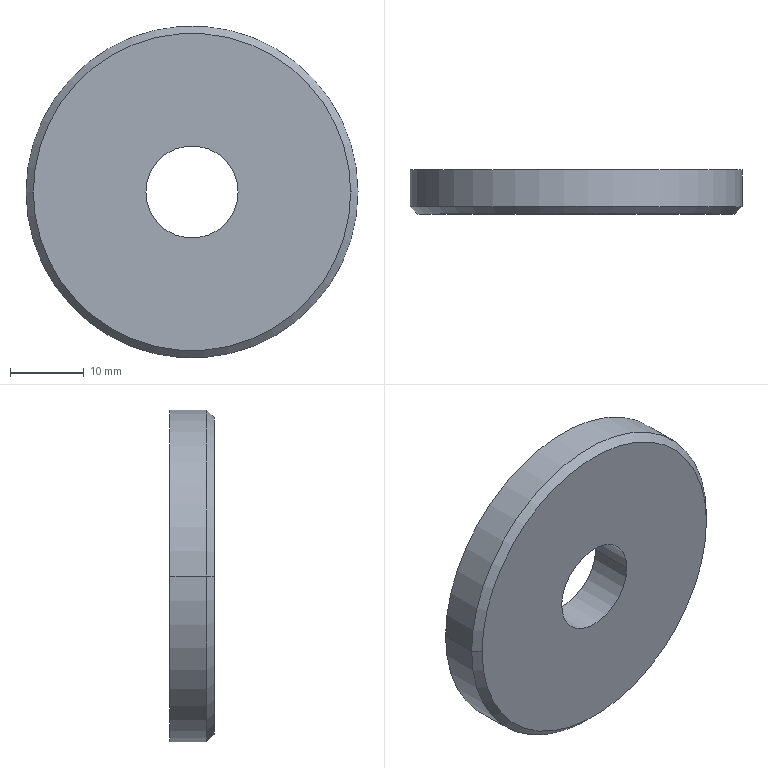Part | SolidWorks | features MBimport 1 | 1 solid | 8 faces | box 45 x 6 x 45 mm | volume 8737 mm3 | cylinder 4 | cone 2 | plane 2 | commonest cylinder face diameters 12.5 x2 45 x2
STEP:
#1=CARTESIAN_POINT('',(22.824,15.416,0.));
#2=VERTEX_POINT('',#1);
#3=CARTESIAN_POINT('',(23.824,16.416,0.));
#4=VERTEX_POINT('',#3);
#5=CARTESIAN_POINT('',(23.824,16.416,0.));
#6=DIRECTION('',(0.7071,0.7071,0.));
#7=VECTOR('',#6,1000.);
#8=LINE('',#5,#7);
#9=EDGE_CURVE('',#2,#4,#8,.T.);
#10=ORIENTED_EDGE('',*,*,#9,.F.);
#11=CARTESIAN_POINT('',(-20.176,15.416,0.));
#12=VERTEX_POINT('',#11);
#13=CARTESIAN_POINT('',(1.324,15.416,0.));
#14=DIRECTION('',(0.,-1.,0.));
#15=DIRECTION('',(1.,0.,0.));
#16=AXIS2_PLACEMENT_3D('',#13,#14,#15);
#17=CIRCLE('',#16,21.5);
#18=EDGE_CURVE('',#12,#2,#17,.T.);
#19=ORIENTED_EDGE('',*,*,#18,.F.);
#20=CARTESIAN_POINT('',(-21.176,16.416,0.));
#21=VERTEX_POINT('',#20);
#22=CARTESIAN_POINT('',(-21.176,16.416,0.));
#23=DIRECTION('',(-0.7071,0.7071,0.));
#24=VECTOR('',#23,1000.);
#25=LINE('',#22,#24);
#26=EDGE_CURVE('',#12,#21,#25,.T.);
#27=ORIENTED_EDGE('',*,*,#26,.T.);
#28=CARTESIAN_POINT('',(1.324,16.416,0.));
#29=DIRECTION('',(0.,1.,0.));
#30=DIRECTION('',(1.,0.,0.));
#31=AXIS2_PLACEMENT_3D('',#28,#29,#30);
#32=CIRCLE('',#31,22.5);
#33=EDGE_CURVE('',#4,#21,#32,.T.);
#34=ORIENTED_EDGE('',*,*,#33,.F.);
#35=EDGE_LOOP('',(#10,#19,#27,#34));
#36=FACE_OUTER_BOUND('',#35,.T.);
#37=CARTESIAN_POINT('',(1.324,16.416,0.));
#38=DIRECTION('',(0.,1.,0.));
#39=DIRECTION('',(-1.,0.,0.));
#40=AXIS2_PLACEMENT_3D('',#37,#38,#39);
#41=CONICAL_SURFACE('',#40,22.5,0.7854);
#42=ADVANCED_FACE('',(#36),#41,.T.);
#43=CARTESIAN_POINT('',(-4.926,21.416,0.));
#44=VERTEX_POINT('',#43);
#45=CARTESIAN_POINT('',(7.574,21.416,0.));
#46=VERTEX_POINT('',#45);
#47=CARTESIAN_POINT('',(1.324,21.416,0.));
#48=DIRECTION('',(0.,1.,0.));
#49=DIRECTION('',(-1.,0.,0.));
#50=AXIS2_PLACEMENT_3D('',#47,#48,#49);
#51=CIRCLE('',#50,6.25);
#52=EDGE_CURVE('',#44,#46,#51,.T.);
#53=ORIENTED_EDGE('',*,*,#52,.F.);
#54=CARTESIAN_POINT('',(1.324,21.416,0.));
#55=DIRECTION('',(0.,1.,0.));
#56=DIRECTION('',(-1.,0.,0.));
#57=AXIS2_PLACEMENT_3D('',#54,#55,#56);
#58=CIRCLE('',#57,6.25);
#59=EDGE_CURVE('',#46,#44,#58,.T.);
#60=ORIENTED_EDGE('',*,*,#59,.F.);
#61=EDGE_LOOP('',(#53,#60));
#62=FACE_BOUND('',#61,.T.);
#63=CARTESIAN_POINT('',(-21.176,21.416,0.));
#64=VERTEX_POINT('',#63);
#65=CARTESIAN_POINT('',(23.824,21.416,0.));
#66=VERTEX_POINT('',#65);
#67=CARTESIAN_POINT('',(1.324,21.416,0.));
#68=DIRECTION('',(0.,1.,0.));
#69=DIRECTION('',(-1.,0.,0.));
#70=AXIS2_PLACEMENT_3D('',#67,#68,#69);
#71=CIRCLE('',#70,22.5);
#72=EDGE_CURVE('',#64,#66,#71,.T.);
#73=ORIENTED_EDGE('',*,*,#72,.T.);
#74=CARTESIAN_POINT('',(1.324,21.416,0.));
#75=DIRECTION('',(0.,1.,0.));
#76=DIRECTION('',(-1.,0.,0.));
#77=AXIS2_PLACEMENT_3D('',#74,#75,#76);
#78=CIRCLE('',#77,22.5);
#79=EDGE_CURVE('',#66,#64,#78,.T.);
#80=ORIENTED_EDGE('',*,*,#79,.T.);
#81=EDGE_LOOP('',(#73,#80));
#82=FACE_OUTER_BOUND('',#81,.T.);
#83=CARTESIAN_POINT('',(-21.176,21.416,0.));
#84=DIRECTION('',(0.,1.,0.));
#85=DIRECTION('',(1.,0.,0.));
#86=AXIS2_PLACEMENT_3D('',#83,#84,#85);
#87=PLANE('',#86);
#88=ADVANCED_FACE('',(#62,#82),#87,.T.);
#89=CARTESIAN_POINT('',(7.574,15.416,0.));
#90=VERTEX_POINT('',#89);
#91=CARTESIAN_POINT('',(7.574,21.416,0.));
#92=DIRECTION('',(0.,1.,0.));
#93=VECTOR('',#92,1000.);
#94=LINE('',#91,#93);
#95=EDGE_CURVE('',#90,#46,#94,.T.);
#96=ORIENTED_EDGE('',*,*,#95,.F.);
#97=CARTESIAN_POINT('',(-4.926,15.416,0.));
#98=VERTEX_POINT('',#97);
#99=CARTESIAN_POINT('',(1.324,15.416,0.));
#100=DIRECTION('',(0.,1.,0.));
#101=DIRECTION('',(-1.,0.,0.));
#102=AXIS2_PLACEMENT_3D('',#99,#100,#101);
#103=CIRCLE('',#102,6.25);
#104=EDGE_CURVE('',#98,#90,#103,.T.);
#105=ORIENTED_EDGE('',*,*,#104,.F.);
#106=CARTESIAN_POINT('',(-4.926,21.416,0.));
#107=DIRECTION('',(0.,1.,0.));
#108=VECTOR('',#107,1000.);
#109=LINE('',#106,#108);
#110=EDGE_CURVE('',#98,#44,#109,.T.);
#111=ORIENTED_EDGE('',*,*,#110,.T.);
#112=ORIENTED_EDGE('',*,*,#52,.T.);
#113=EDGE_LOOP('',(#96,#105,#111,#112));
#114=FACE_OUTER_BOUND('',#113,.T.);
#115=CARTESIAN_POINT('',(1.324,21.416,0.));
#116=DIRECTION('',(0.,1.,0.));
#117=DIRECTION('',(-1.,0.,0.));
#118=AXIS2_PLACEMENT_3D('',#115,#116,#117);
#119=CYLINDRICAL_SURFACE('',#118,6.25);
#120=ADVANCED_FACE('',(#114),#119,.F.);
#121=ORIENTED_EDGE('',*,*,#104,.T.);
#122=CARTESIAN_POINT('',(1.324,15.416,0.));
#123=DIRECTION('',(0.,1.,0.));
#124=DIRECTION('',(-1.,0.,0.));
#125=AXIS2_PLACEMENT_3D('',#122,#123,#124);
#126=CIRCLE('',#125,6.25);
#127=EDGE_CURVE('',#90,#98,#126,.T.);
#128=ORIENTED_EDGE('',*,*,#127,.T.);
#129=EDGE_LOOP('',(#121,#128));
#130=FACE_BOUND('',#129,.T.);
#131=ORIENTED_EDGE('',*,*,#18,.T.);
#132=CARTESIAN_POINT('',(1.324,15.416,0.));
#133=DIRECTION('',(0.,-1.,0.));
#134=DIRECTION('',(1.,0.,0.));
#135=AXIS2_PLACEMENT_3D('',#132,#133,#134);
#136=CIRCLE('',#135,21.5);
#137=EDGE_CURVE('',#2,#12,#136,.T.);
#138=ORIENTED_EDGE('',*,*,#137,.T.);
#139=EDGE_LOOP('',(#131,#138));
#140=FACE_OUTER_BOUND('',#139,.T.);
#141=CARTESIAN_POINT('',(-21.176,15.416,0.));
#142=DIRECTION('',(0.,-1.,0.));
#143=DIRECTION('',(0.,0.,-1.));
#144=AXIS2_PLACEMENT_3D('',#141,#142,#143);
#145=PLANE('',#144);
#146=ADVANCED_FACE('',(#130,#140),#145,.T.);
#147=CARTESIAN_POINT('',(23.824,21.416,0.));
#148=DIRECTION('',(0.,1.,0.));
#149=VECTOR('',#148,1000.);
#150=LINE('',#147,#149);
#151=EDGE_CURVE('',#4,#66,#150,.T.);
#152=ORIENTED_EDGE('',*,*,#151,.F.);
#153=ORIENTED_EDGE('',*,*,#33,.T.);
#154=CARTESIAN_POINT('',(-21.176,21.416,0.));
#155=DIRECTION('',(0.,1.,0.));
#156=VECTOR('',#155,1000.);
#157=LINE('',#154,#156);
#158=EDGE_CURVE('',#21,#64,#157,.T.);
#159=ORIENTED_EDGE('',*,*,#158,.T.);
#160=ORIENTED_EDGE('',*,*,#79,.F.);
#161=EDGE_LOOP('',(#152,#153,#159,#160));
#162=FACE_OUTER_BOUND('',#161,.T.);
#163=CARTESIAN_POINT('',(1.324,21.416,0.));
#164=DIRECTION('',(0.,1.,0.));
#165=DIRECTION('',(-1.,0.,0.));
#166=AXIS2_PLACEMENT_3D('',#163,#164,#165);
#167=CYLINDRICAL_SURFACE('',#166,22.5);
#168=ADVANCED_FACE('',(#162),#167,.T.);
#169=CARTESIAN_POINT('',(1.324,16.416,0.));
#170=DIRECTION('',(0.,1.,0.));
#171=DIRECTION('',(1.,0.,0.));
#172=AXIS2_PLACEMENT_3D('',#169,#170,#171);
#173=CIRCLE('',#172,22.5);
#174=EDGE_CURVE('',#21,#4,#173,.T.);
#175=ORIENTED_EDGE('',*,*,#174,.T.);
#176=ORIENTED_EDGE('',*,*,#151,.T.);
#177=ORIENTED_EDGE('',*,*,#72,.F.);
#178=ORIENTED_EDGE('',*,*,#158,.F.);
#179=EDGE_LOOP('',(#175,#176,#177,#178));
#180=FACE_OUTER_BOUND('',#179,.T.);
#181=CARTESIAN_POINT('',(1.324,21.416,0.));
#182=DIRECTION('',(0.,1.,0.));
#183=DIRECTION('',(-1.,0.,0.));
#184=AXIS2_PLACEMENT_3D('',#181,#182,#183);
#185=CYLINDRICAL_SURFACE('',#184,22.5);
#186=ADVANCED_FACE('',(#180),#185,.T.);
#187=ORIENTED_EDGE('',*,*,#127,.F.);
#188=ORIENTED_EDGE('',*,*,#95,.T.);
#189=ORIENTED_EDGE('',*,*,#59,.T.);
#190=ORIENTED_EDGE('',*,*,#110,.F.);
#191=EDGE_LOOP('',(#187,#188,#189,#190));
#192=FACE_OUTER_BOUND('',#191,.T.);
#193=CARTESIAN_POINT('',(1.324,21.416,0.));
#194=DIRECTION('',(0.,1.,0.));
#195=DIRECTION('',(-1.,0.,0.));
#196=AXIS2_PLACEMENT_3D('',#193,#194,#195);
#197=CYLINDRICAL_SURFACE('',#196,6.25);
#198=ADVANCED_FACE('',(#192),#197,.F.);
#199=ORIENTED_EDGE('',*,*,#137,.F.);
#200=ORIENTED_EDGE('',*,*,#9,.T.);
#201=ORIENTED_EDGE('',*,*,#174,.F.);
#202=ORIENTED_EDGE('',*,*,#26,.F.);
#203=EDGE_LOOP('',(#199,#200,#201,#202));
#204=FACE_OUTER_BOUND('',#203,.T.);
#205=CARTESIAN_POINT('',(1.324,16.416,0.));
#206=DIRECTION('',(0.,1.,0.));
#207=DIRECTION('',(-1.,0.,0.));
#208=AXIS2_PLACEMENT_3D('',#205,#206,#207);
#209=CONICAL_SURFACE('',#208,22.5,0.7854);
#210=ADVANCED_FACE('',(#204),#209,.T.);
#211=CLOSED_SHELL('',(#42,#88,#120,#146,#168,#186,#198,#210));
#212=MANIFOLD_SOLID_BREP('',#211);
#213=CARTESIAN_POINT('',(0.,0.,0.));
#214=DIRECTION('',(0.,0.,1.));
#215=DIRECTION('',(1.,0.,0.));
#216=AXIS2_PLACEMENT_3D('',#213,#214,#215);
#217=(LENGTH_UNIT()NAMED_UNIT(*)SI_UNIT(.MILLI.,.METRE.));
#218=UNCERTAINTY_MEASURE_WITH_UNIT(LENGTH_MEASURE(0.00001),#217,'','');
#219=(NAMED_UNIT(*)PLANE_ANGLE_UNIT()SI_UNIT($,.RADIAN.));
#220=(NAMED_UNIT(*)SI_UNIT($,.STERADIAN.)SOLID_ANGLE_UNIT());
#221=(GEOMETRIC_REPRESENTATION_CONTEXT(3)GLOBAL_UNCERTAINTY_ASSIGNED_CONTEXT((#218))GLOBAL_UNIT_ASSIGNED_CONTEXT((#217,#219,#220))REPRESENTATION_CONTEXT('',''));
#222=ADVANCED_BREP_SHAPE_REPRESENTATION('',(#212,#216),#221);